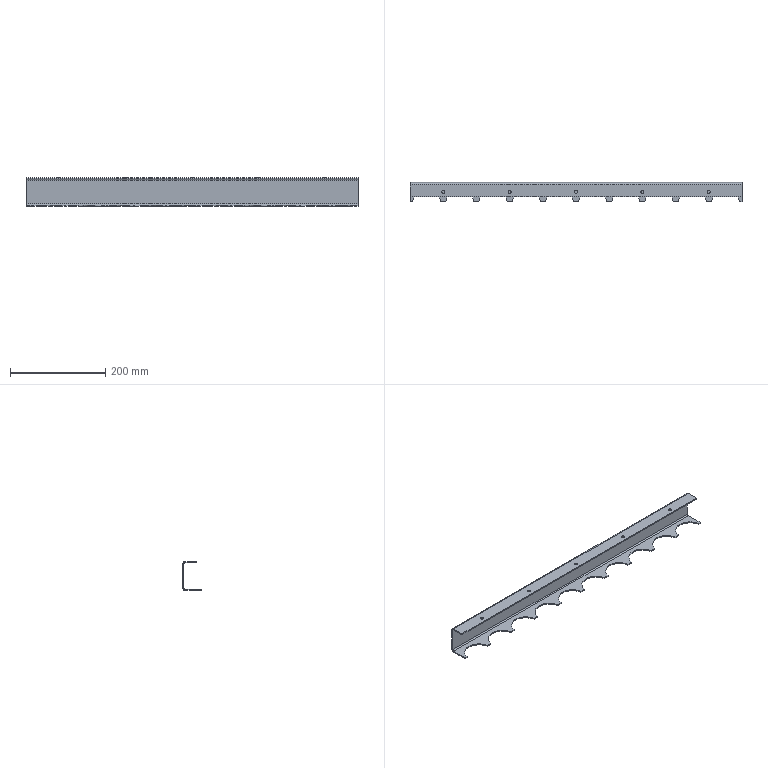Part | STEP file | cc-coverrollers-09 | 1 solid | 39 faces | box 698 x 40 x 60 mm | volume 184215 mm3 | plane 20 | cylinder 14 | spline 5 | commonest cylinder face diameters 60 x10 5 x2 10 x2